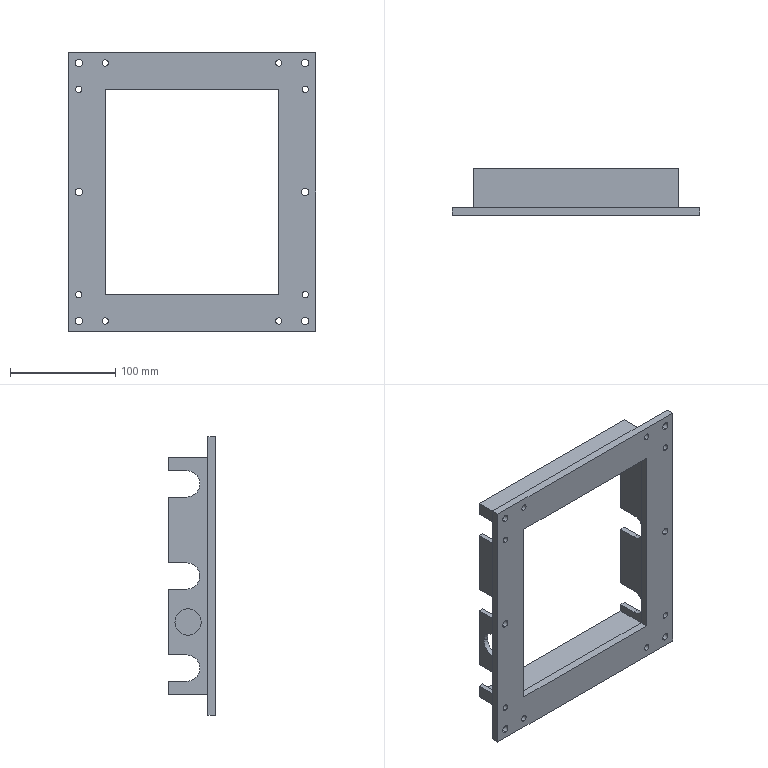Part | STEP file | 2026.6.15-Main Assembly图.sldasm-Part-117 | 1 solid | 85 faces | box 235 x 45 x 265 mm | volume 353113 mm3 | plane 43 | cylinder 42 | commonest cylinder face diameters 6 x16 7 x12 24.9 x12 25 x2